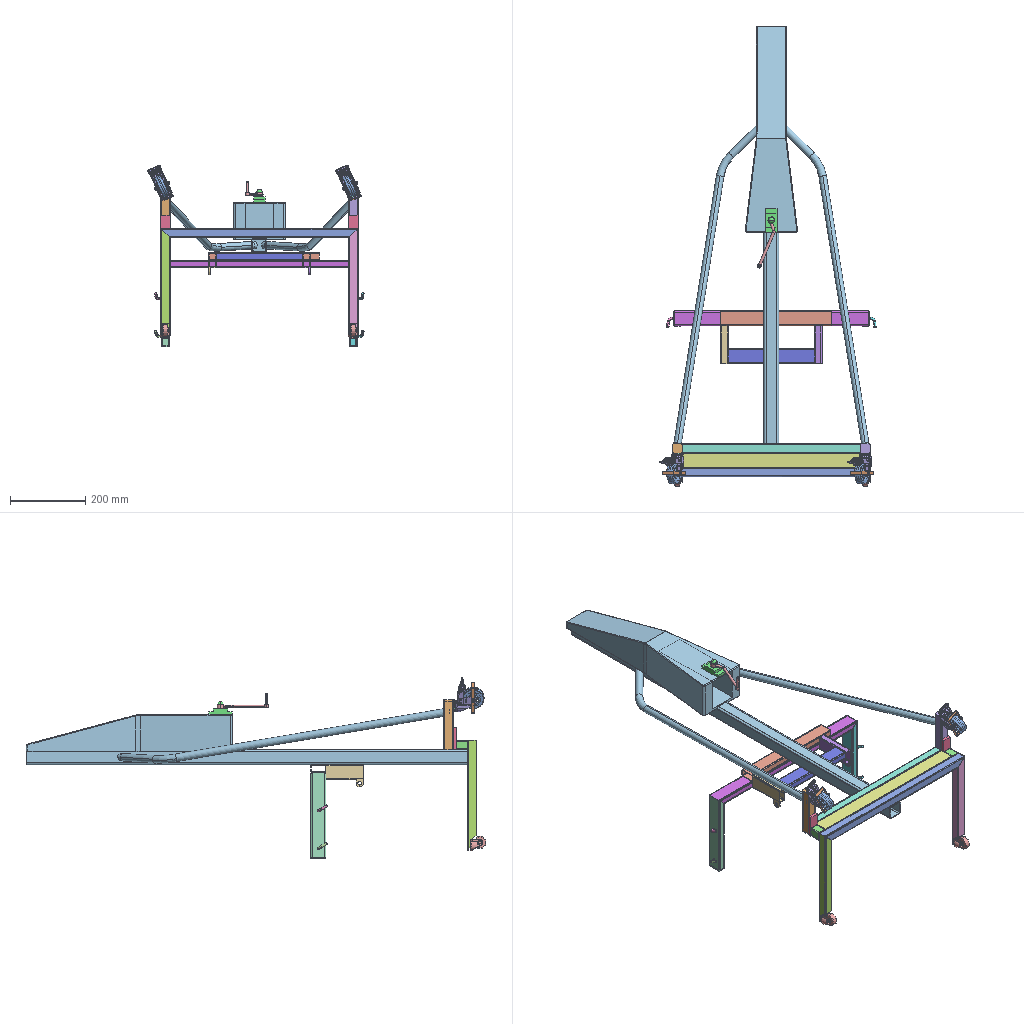Assembly | SolidWorks | 10 different items | 13 placed | box 575 x 1224 x 483 mm
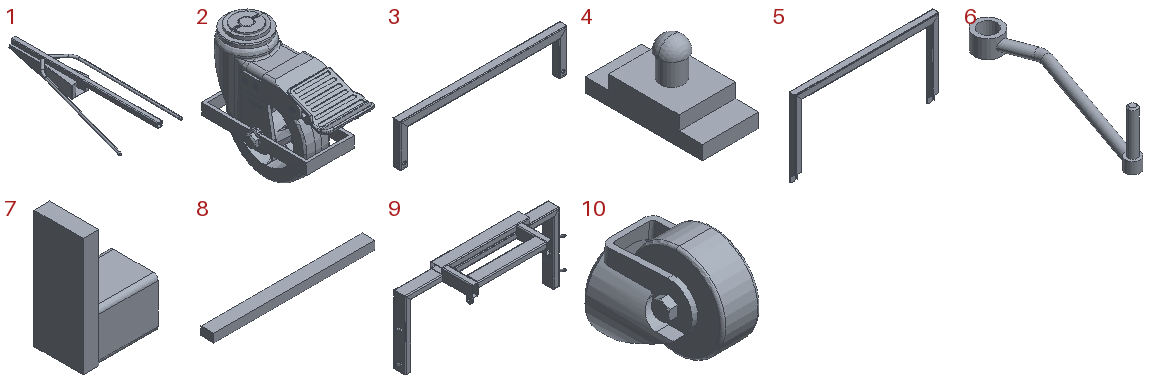Parts list (item | quantity | size | volume | features):
1 | x1 | 524.94 x 1200 x 151.697 mm | 3872299 mm3 | features Fillet 6, ICE 4, 3DProfileFeature 2, MirrorPattern 2, Sweep 1, WeldMemberFeat 1, WeldmentFeature 1
2 | x2 | - | - | features BaseBody 4, ICE 4, RefSurface 1, Scale 1
3 | x1 | 525 x 25 x 132.5 mm | 84662 mm3 | features Cut 1, ICE 1, WeldMemberFeat 1, WeldmentFeature 1
4 | x1 | 30 x 62.5 x 35 mm | 24918 mm3 | features ICE 2, Extrusion 1, Revolution 1, Scale 1
5 | x1 | 525 x 25 x 292.5 mm | 111905 mm3 | features Fillet 2, ICE 2, WeldMemberFeat 1, WeldmentFeature 1
6 | x1 | 40.944 x 138.187 x 40.25 mm | 7860 mm3 | features 3DProfileFeature 2, ICE 2, Chamfer 1, Extrusion 1, Sweep 1
7 | x2 | 38 x 25 x 60 mm | 15316 mm3 | features ICE 1, WeldMemberFeat 1, WeldmentFeature 1
8 | x1 | 475 x 38 x 25 mm | 451250 mm3 | features Extrusion 1
9 | x1 | 557.288 x 140 x 250 mm | 285263 mm3 | features WeldCornerFeat 4, ICE 3, WeldMemberFeat 3, 3DProfileFeature 2, LPattern 1, MirrorPattern 1, Sweep 1, WeldmentFeature 1
10 | x2 | 27.5 x 45 x 38.75 mm | 15003 mm3 | features ICE 3, BaseBody 2
Mates (type | each side: item.copy, entity, surface, feature):
Coincident | 10.1 plane | assembly plane | 3 times
Coincident | 10.1 face plane Input1 | 5.1 face plane Cut-Extrude3
Concentric | 10.1 face cone Input1 | 5.1 face cylinder Fillet1
Parallel | 10.1 face plane Input1 | 5.1 face plane Gb/6728-1986 square hollow section 025 X 25 X 1.2(1)
Parallel | 5.1 face plane Gb/6728-1986 square hollow section 025 X 25 X 1.2(1) | 3.1 face plane Gb/6728-1986 square hollow section 025 X 25 X 1.2(1)
Coincident | 5.1 face plane Gb/6728-1986 square hollow section 025 X 25 X 1.2(1) | 7.1 face plane Gb/6728-1986 square hollow section 025 X 25 X 1.2(1) | 2 times
Coincident | 3.1 face plane Gb/6728-1986 square hollow section 025 X 25 X 1.2(1) | 7.1 face plane Boss-Extrude1 | 2 times
Concentric | 3.1 edge | 2.1 face cylinder Cut-Extrude2
Coincident | 3.1 face plane Gb/6728-1986 square hollow section 025 X 25 X 1.2(1) | 2.1 face plane Input14
Coincident | 7.1 face plane Gb/6728-1986 square hollow section 025 X 25 X 1.2(1) | 8.1 face plane Boss-Extrude1 | 2 times
Coincident | 3.1 face plane Gb/6728-1986 square hollow section 025 X 25 X 1.2(1) | 8.1 face plane Boss-Extrude1
Coincident | 5.1 face plane Gb/6728-1986 square hollow section 025 X 25 X 1.2(1) | 1.1 face plane Gb/6728-1986 square hollow section 040 X 40 X 3(1) | 2 times
Width | 1.1 face plane Gb/6728-1986 square hollow section 040 X 40 X 3(1) | 1.1 face plane Gb/6728-1986 square hollow section 040 X 40 X 3(1) | 5.1 face plane Gb/6728-1986 square hollow section 025 X 25 X 1.2(1) | 5.1 face plane Gb/6728-1986 square hollow section 025 X 25 X 1.2(1)
Width | 9.1 face plane Gb/6728-1986 rectangular hollow section 040 X 20 X 1.5(1) | 9.1 face plane Gb/6728-1986 rectangular hollow section 040 X 20 X 1.5(1) | 5.1 face plane Gb/6728-1986 square hollow section 025 X 25 X 1.2(1) | 5.1 face plane Gb/6728-1986 square hollow section 025 X 25 X 1.2(1)
Coincident | 1.1 face plane Boss-Extrude2 | 4.1 face plane Boss-Extrude1 | 2 times
Width | 4.1 face plane Boss-Extrude1 | 4.1 face plane Boss-Extrude1 | 1.1 face plane Boss-Extrude2 | 1.1 face plane Boss-Extrude2
Concentric | 4.1 face cylinder Boss-Extrude3 | 6.1 face cylinder Boss-Extrude1
Coincident | 4.1 face plane Boss-Extrude2 | 6.1 face plane Boss-Extrude1
Coincident | 5.1 face plane Gb/6728-1986 square hollow section 025 X 25 X 1.2(1) | 3.1 face plane Gb/6728-1986 square hollow section 025 X 25 X 1.2(1) | 2 times
Coincident | 1.1 face plane Gb/6728-1986 square hollow section 040 X 40 X 3(1) | 9.1 face plane Gb/6728-1986 rectangular hollow section 040 X 20 X 1.5(6)